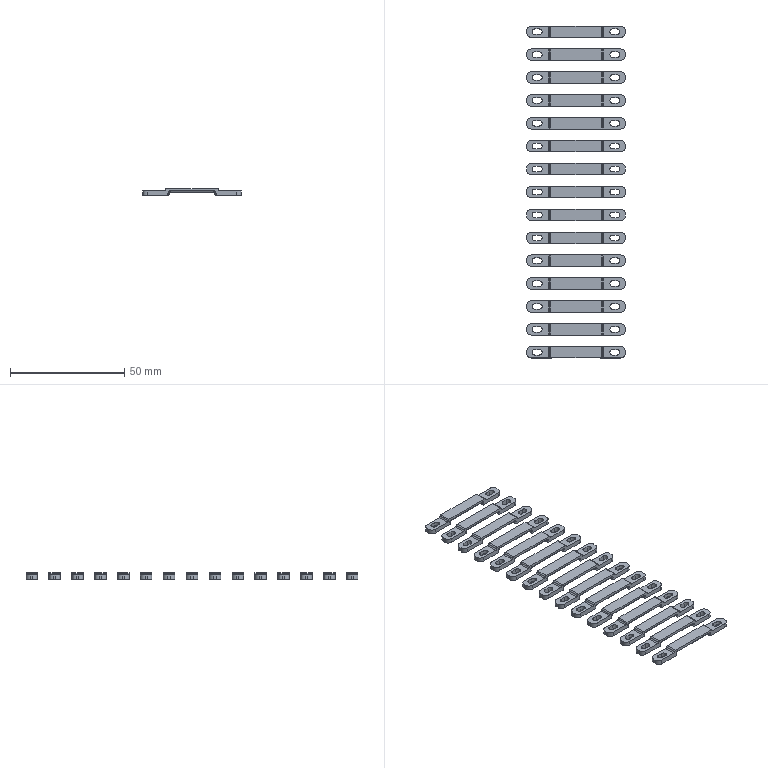NC program | NX | posted with a generic post | part box 43 x 145 x 3 mm
Lines 19 to 1188 of 17881:
(ZLEVEL_PROFILE , TOOL : D4)
N36 T11 M6
N38 G54
N40 G17 G0 G90 X65.4 Y-2.835 S9500 M3
N42 G43 Z30. H11
N44 Z1.5
N46 G94 G1 Y19.997 Z0.303 F1000.
N48 X65.787 Y21.308 Z0.232
N50 X66.58 Y22.42 Z0.16
N52 X67.692 Y23.213 Z0.089
N54 X69.003 Y23.6 Z0.017
N56 X70.997 Z-0.088
N58 X72.308 Y23.213 Z-0.159
N60 X73.42 Y22.42 Z-0.231
N62 X74.213 Y21.308 Z-0.302
N64 X74.6 Y19.997 Z-0.374
N66 Y19.5 Z-0.4
N68 Y-19.5 F2500.
N70 G2 X70.5 Y-23.6 R4.1
N72 G1 X69.5
N74 G2 X65.4 Y-19.5 R4.1
N76 G1 Y19.5
N78 G2 X69.5 Y23.6 R4.1
N80 G1 X70.5
N82 G2 X74.6 Y19.5 R4.1
N84 G1 Y-3.416 Z-0.8
N86 Y-19.5
N88 G2 X70.5 Y-23.6 R4.1
N90 G1 X69.5
N92 G2 X65.4 Y-19.5 R4.1
N94 G1 Y19.5
N96 G2 X69.5 Y23.6 R4.1
N98 G1 X70.5
N100 G2 X74.6 Y19.5 R4.1
N102 G1 Y-3.416 Z-1.2
N104 Y-19.5
N106 G2 X70.5 Y-23.6 R4.1
N108 G1 X69.5
N110 G2 X65.4 Y-19.5 R4.1
N112 G1 Y19.5
N114 G2 X69.5 Y23.6 R4.1
N116 G1 X70.5
N118 G2 X74.6 Y19.5 R4.1
N120 G1 Y-3.416 Z-1.6
N122 Y-19.5
N124 G2 X70.5 Y-23.6 R4.1
N126 G1 X69.5
N128 G2 X65.4 Y-19.5 R4.1
N130 G1 Y19.5
N132 G2 X69.5 Y23.6 R4.1
N134 G1 X70.5
N136 G2 X74.6 Y19.5 R4.1
N138 G1 Y-3.416 Z-2.
N140 Y-19.5
N142 G2 X70.5 Y-23.6 R4.1
N144 G1 X69.5
N146 G2 X65.4 Y-19.5 R4.1
N148 G1 Y19.5
N150 G2 X69.5 Y23.6 R4.1
N152 G1 X70.5
N154 G2 X74.6 Y19.5 R4.1
N156 G1 Y-3.416 Z-2.4
N158 Y-19.5
N160 G2 X70.5 Y-23.6 R4.1
N162 G1 X69.5
N164 G2 X65.4 Y-19.5 R4.1
N166 G1 Y19.5
N168 G2 X69.5 Y23.6 R4.1
N170 G1 X70.5
N172 G2 X74.6 Y19.5 R4.1
N174 G1 Y-3.416
N176 Z-0.9
N178 G0 Z30.
N180 X55.4 Y-2.835
N182 Z1.5
N184 G1 Y19.997 Z0.303 F1000.
N186 X55.787 Y21.308 Z0.232
N188 X56.58 Y22.42 Z0.16
N190 X57.692 Y23.213 Z0.089
N192 X59.003 Y23.6 Z0.017
N194 X60.997 Z-0.088
N196 X62.308 Y23.213 Z-0.159
N198 X63.42 Y22.42 Z-0.231
N200 X64.213 Y21.308 Z-0.302
N202 X64.6 Y19.997 Z-0.374
N204 Y19.5 Z-0.4
N206 Y-19.5 F2500.
N208 G2 X60.5 Y-23.6 R4.1
N210 G1 X59.5
N212 G2 X55.4 Y-19.5 R4.1
N214 G1 Y19.5
N216 G2 X59.5 Y23.6 R4.1
N218 G1 X60.5
N220 G2 X64.6 Y19.5 R4.1
N222 G1 Y-3.416 Z-0.8
N224 Y-19.5
N226 G2 X60.5 Y-23.6 R4.1
N228 G1 X59.5
N230 G2 X55.4 Y-19.5 R4.1
N232 G1 Y19.5
N234 G2 X59.5 Y23.6 R4.1
N236 G1 X60.5
N238 G2 X64.6 Y19.5 R4.1
N240 G1 Y-3.416 Z-1.2
N242 Y-19.5
N244 G2 X60.5 Y-23.6 R4.1
N246 G1 X59.5
N248 G2 X55.4 Y-19.5 R4.1
N250 G1 Y19.5
N252 G2 X59.5 Y23.6 R4.1
N254 G1 X60.5
N256 G2 X64.6 Y19.5 R4.1
N258 G1 Y-3.416 Z-1.6
N260 Y-19.5
N262 G2 X60.5 Y-23.6 R4.1
N264 G1 X59.5
N266 G2 X55.4 Y-19.5 R4.1
N268 G1 Y19.5
N270 G2 X59.5 Y23.6 R4.1
N272 G1 X60.5
N274 G2 X64.6 Y19.5 R4.1
N276 G1 Y-3.416 Z-2.
N278 Y-19.5
N280 G2 X60.5 Y-23.6 R4.1
N282 G1 X59.5
N284 G2 X55.4 Y-19.5 R4.1
N286 G1 Y19.5
N288 G2 X59.5 Y23.6 R4.1
N290 G1 X60.5
N292 G2 X64.6 Y19.5 R4.1
N294 G1 Y-3.416 Z-2.4
N296 Y-19.5
N298 G2 X60.5 Y-23.6 R4.1
N300 G1 X59.5
N302 G2 X55.4 Y-19.5 R4.1
N304 G1 Y19.5
N306 G2 X59.5 Y23.6 R4.1
N308 G1 X60.5
N310 G2 X64.6 Y19.5 R4.1
N312 G1 Y-3.416
N314 Z-0.9
N316 G0 Z30.
N318 X45.4 Y-2.835
N320 Z1.5
N322 G1 Y19.997 Z0.303 F1000.
N324 X45.787 Y21.308 Z0.232
N326 X46.58 Y22.42 Z0.16
N328 X47.692 Y23.213 Z0.089
N330 X49.003 Y23.6 Z0.017
N332 X50.997 Z-0.088
N334 X52.308 Y23.213 Z-0.159
N336 X53.42 Y22.42 Z-0.231
N338 X54.213 Y21.308 Z-0.302
N340 X54.6 Y19.997 Z-0.374
N342 Y19.5 Z-0.4
N344 Y-19.5 F2500.
N346 G2 X50.5 Y-23.6 R4.1
N348 G1 X49.5
N350 G2 X45.4 Y-19.5 R4.1
N352 G1 Y19.5
N354 G2 X49.5 Y23.6 R4.1
N356 G1 X50.5
N358 G2 X54.6 Y19.5 R4.1
N360 G1 Y-3.416 Z-0.8
N362 Y-19.5
N364 G2 X50.5 Y-23.6 R4.1
N366 G1 X49.5
N368 G2 X45.4 Y-19.5 R4.1
N370 G1 Y19.5
N372 G2 X49.5 Y23.6 R4.1
N374 G1 X50.5
N376 G2 X54.6 Y19.5 R4.1
N378 G1 Y-3.416 Z-1.2
N380 Y-19.5
N382 G2 X50.5 Y-23.6 R4.1
N384 G1 X49.5
N386 G2 X45.4 Y-19.5 R4.1
N388 G1 Y19.5
N390 G2 X49.5 Y23.6 R4.1
N392 G1 X50.5
N394 G2 X54.6 Y19.5 R4.1
N396 G1 Y-3.416 Z-1.6
N398 Y-19.5
N400 G2 X50.5 Y-23.6 R4.1
N402 G1 X49.5
N404 G2 X45.4 Y-19.5 R4.1
N406 G1 Y19.5
N408 G2 X49.5 Y23.6 R4.1
N410 G1 X50.5
N412 G2 X54.6 Y19.5 R4.1
N414 G1 Y-3.416 Z-2.
N416 Y-19.5
N418 G2 X50.5 Y-23.6 R4.1
N420 G1 X49.5
N422 G2 X45.4 Y-19.5 R4.1
N424 G1 Y19.5
N426 G2 X49.5 Y23.6 R4.1
N428 G1 X50.5
N430 G2 X54.6 Y19.5 R4.1
N432 G1 Y-3.416 Z-2.4
N434 Y-19.5
N436 G2 X50.5 Y-23.6 R4.1
N438 G1 X49.5
N440 G2 X45.4 Y-19.5 R4.1
N442 G1 Y19.5
N444 G2 X49.5 Y23.6 R4.1
N446 G1 X50.5
N448 G2 X54.6 Y19.5 R4.1
N450 G1 Y-3.416
N452 Z-0.9
N454 G0 Z30.
N456 X35.4 Y-2.835
N458 Z1.5
N460 G1 Y19.997 Z0.303 F1000.
N462 X35.787 Y21.308 Z0.232
N464 X36.58 Y22.42 Z0.16
N466 X37.692 Y23.213 Z0.089
N468 X39.003 Y23.6 Z0.017
N470 X40.997 Z-0.088
N472 X42.308 Y23.213 Z-0.159
N474 X43.42 Y22.42 Z-0.231
N476 X44.213 Y21.308 Z-0.302
N478 X44.6 Y19.997 Z-0.374
N480 Y19.5 Z-0.4
N482 Y-19.5 F2500.
N484 G2 X40.5 Y-23.6 R4.1
N486 G1 X39.5
N488 G2 X35.4 Y-19.5 R4.1
N490 G1 Y19.5
N492 G2 X39.5 Y23.6 R4.1
N494 G1 X40.5
N496 G2 X44.6 Y19.5 R4.1
N498 G1 Y-3.416 Z-0.8
N500 Y-19.5
N502 G2 X40.5 Y-23.6 R4.1
N504 G1 X39.5
N506 G2 X35.4 Y-19.5 R4.1
N508 G1 Y19.5
N510 G2 X39.5 Y23.6 R4.1
N512 G1 X40.5
N514 G2 X44.6 Y19.5 R4.1
N516 G1 Y-3.416 Z-1.2
N518 Y-19.5
N520 G2 X40.5 Y-23.6 R4.1
N522 G1 X39.5
N524 G2 X35.4 Y-19.5 R4.1
N526 G1 Y19.5
N528 G2 X39.5 Y23.6 R4.1
N530 G1 X40.5
N532 G2 X44.6 Y19.5 R4.1
N534 G1 Y-3.416 Z-1.6
N536 Y-19.5
N538 G2 X40.5 Y-23.6 R4.1
N540 G1 X39.5
N542 G2 X35.4 Y-19.5 R4.1
N544 G1 Y19.5
N546 G2 X39.5 Y23.6 R4.1
N548 G1 X40.5
N550 G2 X44.6 Y19.5 R4.1
N552 G1 Y-3.416 Z-2.
N554 Y-19.5
N556 G2 X40.5 Y-23.6 R4.1
N558 G1 X39.5
N560 G2 X35.4 Y-19.5 R4.1
N562 G1 Y19.5
N564 G2 X39.5 Y23.6 R4.1
N566 G1 X40.5
N568 G2 X44.6 Y19.5 R4.1
N570 G1 Y-3.416 Z-2.4
N572 Y-19.5
N574 G2 X40.5 Y-23.6 R4.1
N576 G1 X39.5
N578 G2 X35.4 Y-19.5 R4.1
N580 G1 Y19.5
N582 G2 X39.5 Y23.6 R4.1
N584 G1 X40.5
N586 G2 X44.6 Y19.5 R4.1
N588 G1 Y-3.416
N590 Z-0.9
N592 G0 Z30.
N594 X25.4 Y-2.835
N596 Z1.5
N598 G1 Y19.997 Z0.303 F1000.
N600 X25.787 Y21.308 Z0.232
N602 X26.58 Y22.42 Z0.16
N604 X27.692 Y23.213 Z0.089
N606 X29.003 Y23.6 Z0.017
N608 X30.997 Z-0.088
N610 X32.308 Y23.213 Z-0.159
N612 X33.42 Y22.42 Z-0.231
N614 X34.213 Y21.308 Z-0.302
N616 X34.6 Y19.997 Z-0.374
N618 Y19.5 Z-0.4
N620 Y-19.5 F2500.
N622 G2 X30.5 Y-23.6 R4.1
N624 G1 X29.5
N626 G2 X25.4 Y-19.5 R4.1
N628 G1 Y19.5
N630 G2 X29.5 Y23.6 R4.1
N632 G1 X30.5
N634 G2 X34.6 Y19.5 R4.1
N636 G1 Y-3.416 Z-0.8
N638 Y-19.5
N640 G2 X30.5 Y-23.6 R4.1
N642 G1 X29.5
N644 G2 X25.4 Y-19.5 R4.1
N646 G1 Y19.5
N648 G2 X29.5 Y23.6 R4.1
N650 G1 X30.5
N652 G2 X34.6 Y19.5 R4.1
N654 G1 Y-3.416 Z-1.2
N656 Y-19.5
N658 G2 X30.5 Y-23.6 R4.1
N660 G1 X29.5
N662 G2 X25.4 Y-19.5 R4.1
N664 G1 Y19.5
N666 G2 X29.5 Y23.6 R4.1
N668 G1 X30.5
N670 G2 X34.6 Y19.5 R4.1
N672 G1 Y-3.416 Z-1.6
N674 Y-19.5
N676 G2 X30.5 Y-23.6 R4.1
N678 G1 X29.5
N680 G2 X25.4 Y-19.5 R4.1
N682 G1 Y19.5
N684 G2 X29.5 Y23.6 R4.1
N686 G1 X30.5
N688 G2 X34.6 Y19.5 R4.1
N690 G1 Y-3.416 Z-2.
N692 Y-19.5
N694 G2 X30.5 Y-23.6 R4.1
N696 G1 X29.5
N698 G2 X25.4 Y-19.5 R4.1
N700 G1 Y19.5
N702 G2 X29.5 Y23.6 R4.1
N704 G1 X30.5
N706 G2 X34.6 Y19.5 R4.1
N708 G1 Y-3.416 Z-2.4
N710 Y-19.5
N712 G2 X30.5 Y-23.6 R4.1
N714 G1 X29.5
N716 G2 X25.4 Y-19.5 R4.1
N718 G1 Y19.5
N720 G2 X29.5 Y23.6 R4.1
N722 G1 X30.5
N724 G2 X34.6 Y19.5 R4.1
N726 G1 Y-3.416
N728 Z-0.9
N730 G0 Z30.
N732 X-44.6 Y-2.835
N734 Z1.5
N736 G1 Y19.997 Z0.303 F1000.
N738 X-44.213 Y21.308 Z0.232
N740 X-43.42 Y22.42 Z0.16
N742 X-42.308 Y23.213 Z0.089
N744 X-40.997 Y23.6 Z0.017
N746 X-39.003 Z-0.088
N748 X-37.692 Y23.213 Z-0.159
N750 X-36.58 Y22.42 Z-0.231
N752 X-35.787 Y21.308 Z-0.302
N754 X-35.4 Y19.997 Z-0.374
N756 Y19.5 Z-0.4
N758 Y-19.5 F2500.
N760 G2 X-39.5 Y-23.6 R4.1
N762 G1 X-40.5
N764 G2 X-44.6 Y-19.5 R4.1
N766 G1 Y19.5
N768 G2 X-40.5 Y23.6 R4.1
N770 G1 X-39.5
N772 G2 X-35.4 Y19.5 R4.1
N774 G1 Y-3.416 Z-0.8
N776 Y-19.5
N778 G2 X-39.5 Y-23.6 R4.1
N780 G1 X-40.5
N782 G2 X-44.6 Y-19.5 R4.1
N784 G1 Y19.5
N786 G2 X-40.5 Y23.6 R4.1
N788 G1 X-39.5
N790 G2 X-35.4 Y19.5 R4.1
N792 G1 Y-3.416 Z-1.2
N794 Y-19.5
N796 G2 X-39.5 Y-23.6 R4.1
N798 G1 X-40.5
N800 G2 X-44.6 Y-19.5 R4.1
N802 G1 Y19.5
N804 G2 X-40.5 Y23.6 R4.1
N806 G1 X-39.5
N808 G2 X-35.4 Y19.5 R4.1
N810 G1 Y-3.416 Z-1.6
N812 Y-19.5
N814 G2 X-39.5 Y-23.6 R4.1
N816 G1 X-40.5
N818 G2 X-44.6 Y-19.5 R4.1
N820 G1 Y19.5
N822 G2 X-40.5 Y23.6 R4.1
N824 G1 X-39.5
N826 G2 X-35.4 Y19.5 R4.1
N828 G1 Y-3.416 Z-2.
N830 Y-19.5
N832 G2 X-39.5 Y-23.6 R4.1
N834 G1 X-40.5
N836 G2 X-44.6 Y-19.5 R4.1
N838 G1 Y19.5
N840 G2 X-40.5 Y23.6 R4.1
N842 G1 X-39.5
N844 G2 X-35.4 Y19.5 R4.1
N846 G1 Y-3.416 Z-2.4
N848 Y-19.5
N850 G2 X-39.5 Y-23.6 R4.1
N852 G1 X-40.5
N854 G2 X-44.6 Y-19.5 R4.1
N856 G1 Y19.5
N858 G2 X-40.5 Y23.6 R4.1
N860 G1 X-39.5
N862 G2 X-35.4 Y19.5 R4.1
N864 G1 Y-3.416
N866 Z-0.9
N868 G0 Z30.
N870 X-55.4 Y2.835
N872 Z1.5
N874 G1 Y-19.997 Z0.303 F1000.
N876 X-55.787 Y-21.308 Z0.232
N878 X-56.58 Y-22.42 Z0.16
N880 X-57.692 Y-23.213 Z0.089
N882 X-59.003 Y-23.6 Z0.017
N884 X-60.997 Z-0.088
N886 X-62.308 Y-23.213 Z-0.159
N888 X-63.42 Y-22.42 Z-0.231
N890 X-64.213 Y-21.308 Z-0.302
N892 X-64.6 Y-19.997 Z-0.374
N894 Y-19.5 Z-0.4
N896 Y19.5 F2500.
N898 G2 X-60.5 Y23.6 R4.1
N900 G1 X-59.5
N902 G2 X-55.4 Y19.5 R4.1
N904 G1 Y-19.5
N906 G2 X-59.5 Y-23.6 R4.1
N908 G1 X-60.5
N910 G2 X-64.6 Y-19.5 R4.1
N912 G1 Y3.416 Z-0.8
N914 Y19.5
N916 G2 X-60.5 Y23.6 R4.1
N918 G1 X-59.5
N920 G2 X-55.4 Y19.5 R4.1
N922 G1 Y-19.5
N924 G2 X-59.5 Y-23.6 R4.1
N926 G1 X-60.5
N928 G2 X-64.6 Y-19.5 R4.1
N930 G1 Y3.416 Z-1.2
N932 Y19.5
N934 G2 X-60.5 Y23.6 R4.1
N936 G1 X-59.5
N938 G2 X-55.4 Y19.5 R4.1
N940 G1 Y-19.5
N942 G2 X-59.5 Y-23.6 R4.1
N944 G1 X-60.5
N946 G2 X-64.6 Y-19.5 R4.1
N948 G1 Y3.416 Z-1.6
N950 Y19.5
N952 G2 X-60.5 Y23.6 R4.1
N954 G1 X-59.5
N956 G2 X-55.4 Y19.5 R4.1
N958 G1 Y-19.5
N960 G2 X-59.5 Y-23.6 R4.1
N962 G1 X-60.5
N964 G2 X-64.6 Y-19.5 R4.1
N966 G1 Y3.416 Z-2.
N968 Y19.5
N970 G2 X-60.5 Y23.6 R4.1
N972 G1 X-59.5
N974 G2 X-55.4 Y19.5 R4.1
N976 G1 Y-19.5
N978 G2 X-59.5 Y-23.6 R4.1
N980 G1 X-60.5
N982 G2 X-64.6 Y-19.5 R4.1
N984 G1 Y3.416 Z-2.4
N986 Y19.5
N988 G2 X-60.5 Y23.6 R4.1
N990 G1 X-59.5
N992 G2 X-55.4 Y19.5 R4.1
N994 G1 Y-19.5
N996 G2 X-59.5 Y-23.6 R4.1
N998 G1 X-60.5
N1000 G2 X-64.6 Y-19.5 R4.1
N1002 G1 Y3.416
N1004 Z-0.9
N1006 G0 Z30.
N1008 X24.6 Y2.835
N1010 Z1.5
N1012 G1 Y-19.997 Z0.303 F1000.
N1014 X24.213 Y-21.308 Z0.232
N1016 X23.42 Y-22.42 Z0.16
N1018 X22.308 Y-23.213 Z0.089
N1020 X20.997 Y-23.6 Z0.017
N1022 X19.003 Z-0.088
N1024 X17.692 Y-23.213 Z-0.159
N1026 X16.58 Y-22.42 Z-0.231
N1028 X15.787 Y-21.308 Z-0.302
N1030 X15.4 Y-19.997 Z-0.374
N1032 Y-19.5 Z-0.4
N1034 Y19.5 F2500.
N1036 G2 X19.5 Y23.6 R4.1
N1038 G1 X20.5
N1040 G2 X24.6 Y19.5 R4.1
N1042 G1 Y-19.5
N1044 G2 X20.5 Y-23.6 R4.1
N1046 G1 X19.5
N1048 G2 X15.4 Y-19.5 R4.1
N1050 G1 Y3.416 Z-0.8
N1052 Y19.5
N1054 G2 X19.5 Y23.6 R4.1
N1056 G1 X20.5
N1058 G2 X24.6 Y19.5 R4.1
N1060 G1 Y-19.5
N1062 G2 X20.5 Y-23.6 R4.1
N1064 G1 X19.5
N1066 G2 X15.4 Y-19.5 R4.1
N1068 G1 Y3.416 Z-1.2
N1070 Y19.5
N1072 G2 X19.5 Y23.6 R4.1
N1074 G1 X20.5
N1076 G2 X24.6 Y19.5 R4.1
N1078 G1 Y-19.5
N1080 G2 X20.5 Y-23.6 R4.1
N1082 G1 X19.5
N1084 G2 X15.4 Y-19.5 R4.1
N1086 G1 Y3.416 Z-1.6
N1088 Y19.5
N1090 G2 X19.5 Y23.6 R4.1
N1092 G1 X20.5
N1094 G2 X24.6 Y19.5 R4.1
N1096 G1 Y-19.5
N1098 G2 X20.5 Y-23.6 R4.1
N1100 G1 X19.5
N1102 G2 X15.4 Y-19.5 R4.1
N1104 G1 Y3.416 Z-2.
N1106 Y19.5
N1108 G2 X19.5 Y23.6 R4.1
N1110 G1 X20.5
N1112 G2 X24.6 Y19.5 R4.1
N1114 G1 Y-19.5
N1116 G2 X20.5 Y-23.6 R4.1
N1118 G1 X19.5
N1120 G2 X15.4 Y-19.5 R4.1
N1122 G1 Y3.416 Z-2.4
N1124 Y19.5
N1126 G2 X19.5 Y23.6 R4.1
N1128 G1 X20.5
N1130 G2 X24.6 Y19.5 R4.1
N1132 G1 Y-19.5
N1134 G2 X20.5 Y-23.6 R4.1
N1136 G1 X19.5
N1138 G2 X15.4 Y-19.5 R4.1
N1140 G1 Y3.416
N1142 Z-0.9
N1144 G0 Z30.
N1146 X-65.4 Y2.835
N1148 Z1.5
N1150 G1 Y-19.997 Z0.303 F1000.
N1152 X-65.787 Y-21.308 Z0.232
N1154 X-66.58 Y-22.42 Z0.16
N1156 X-67.692 Y-23.213 Z0.089
N1158 X-69.003 Y-23.6 Z0.017
N1160 X-70.997 Z-0.088
N1162 X-72.308 Y-23.213 Z-0.159
N1164 X-73.42 Y-22.42 Z-0.231
N1166 X-74.213 Y-21.308 Z-0.302
N1168 X-74.6 Y-19.997 Z-0.374
N1170 Y-19.5 Z-0.4
N1172 Y19.5 F2500.
N1174 G2 X-70.5 Y23.6 R4.1
N1176 G1 X-69.5
N1178 G2 X-65.4 Y19.5 R4.1
N1180 G1 Y-19.5
N1182 G2 X-69.5 Y-23.6 R4.1
N1184 G1 X-70.5
N1186 G2 X-74.6 Y-19.5 R4.1
N1188 G1 Y3.416 Z-0.8
N1190 Y19.5
N1192 G2 X-70.5 Y23.6 R4.1
N1194 G1 X-69.5
N1196 G2 X-65.4 Y19.5 R4.1
N1198 G1 Y-19.5
N1200 G2 X-69.5 Y-23.6 R4.1
N1202 G1 X-70.5
N1204 G2 X-74.6 Y-19.5 R4.1
N1206 G1 Y3.416 Z-1.2
N1208 Y19.5
N1210 G2 X-70.5 Y23.6 R4.1
N1212 G1 X-69.5
N1214 G2 X-65.4 Y19.5 R4.1
N1216 G1 Y-19.5
N1218 G2 X-69.5 Y-23.6 R4.1
N1220 G1 X-70.5
N1222 G2 X-74.6 Y-19.5 R4.1
N1224 G1 Y3.416 Z-1.6
N1226 Y19.5
N1228 G2 X-70.5 Y23.6 R4.1
N1230 G1 X-69.5
N1232 G2 X-65.4 Y19.5 R4.1
N1234 G1 Y-19.5
N1236 G2 X-69.5 Y-23.6 R4.1
N1238 G1 X-70.5
N1240 G2 X-74.6 Y-19.5 R4.1
N1242 G1 Y3.416 Z-2.
N1244 Y19.5
N1246 G2 X-70.5 Y23.6 R4.1
N1248 G1 X-69.5
N1250 G2 X-65.4 Y19.5 R4.1
N1252 G1 Y-19.5
N1254 G2 X-69.5 Y-23.6 R4.1
N1256 G1 X-70.5
N1258 G2 X-74.6 Y-19.5 R4.1
N1260 G1 Y3.416 Z-2.4
N1262 Y19.5
N1264 G2 X-70.5 Y23.6 R4.1
N1266 G1 X-69.5
N1268 G2 X-65.4 Y19.5 R4.1
N1270 G1 Y-19.5
N1272 G2 X-69.5 Y-23.6 R4.1
N1274 G1 X-70.5
N1276 G2 X-74.6 Y-19.5 R4.1
N1278 G1 Y3.416
N1280 Z-0.9
N1282 G0 Z30.
N1284 X14.6 Y2.835
N1286 Z1.5
N1288 G1 Y-19.997 Z0.303 F1000.
N1290 X14.213 Y-21.308 Z0.232
N1292 X13.42 Y-22.42 Z0.16
N1294 X12.308 Y-23.213 Z0.089
N1296 X10.997 Y-23.6 Z0.017
N1298 X9.003 Z-0.088
N1300 X7.692 Y-23.213 Z-0.159
N1302 X6.58 Y-22.42 Z-0.231
N1304 X5.787 Y-21.308 Z-0.302
N1306 X5.4 Y-19.997 Z-0.374
N1308 Y-19.5 Z-0.4
N1310 Y19.5 F2500.
N1312 G2 X9.5 Y23.6 R4.1
N1314 G1 X10.5
N1316 G2 X14.6 Y19.5 R4.1
N1318 G1 Y-19.5
N1320 G2 X10.5 Y-23.6 R4.1
N1322 G1 X9.5
N1324 G2 X5.4 Y-19.5 R4.1
N1326 G1 Y3.416 Z-0.8
N1328 Y19.5
N1330 G2 X9.5 Y23.6 R4.1
N1332 G1 X10.5
N1334 G2 X14.6 Y19.5 R4.1
N1336 G1 Y-19.5
N1338 G2 X10.5 Y-23.6 R4.1
N1340 G1 X9.5
N1342 G2 X5.4 Y-19.5 R4.1
N1344 G1 Y3.416 Z-1.2
N1346 Y19.5
N1348 G2 X9.5 Y23.6 R4.1
N1350 G1 X10.5
N1352 G2 X14.6 Y19.5 R4.1
N1354 G1 Y-19.5
N1356 G2 X10.5 Y-23.6 R4.1
N1358 G1 X9.5
N1360 G2 X5.4 Y-19.5 R4.1
N1362 G1 Y3.416 Z-1.6
N1364 Y19.5
N1366 G2 X9.5 Y23.6 R4.1
N1368 G1 X10.5
N1370 G2 X14.6 Y19.5 R4.1
N1372 G1 Y-19.5
N1374 G2 X10.5 Y-23.6 R4.1
N1376 G1 X9.5
N1378 G2 X5.4 Y-19.5 R4.1
N1380 G1 Y3.416 Z-2.
N1382 Y19.5
N1384 G2 X9.5 Y23.6 R4.1
N1386 G1 X10.5
N1388 G2 X14.6 Y19.5 R4.1
N1390 G1 Y-19.5
N1392 G2 X10.5 Y-23.6 R4.1
N1394 G1 X9.5
N1396 G2 X5.4 Y-19.5 R4.1
N1398 G1 Y3.416 Z-2.4
N1400 Y19.5
N1402 G2 X9.5 Y23.6 R4.1
N1404 G1 X10.5
N1406 G2 X14.6 Y19.5 R4.1
N1408 G1 Y-19.5
N1410 G2 X10.5 Y-23.6 R4.1
N1412 G1 X9.5
N1414 G2 X5.4 Y-19.5 R4.1
N1416 G1 Y3.416
N1418 Z-0.9
N1420 G0 Z30.
N1422 X-4.6 Y-2.835
N1424 Z1.5
N1426 G1 Y19.997 Z0.303 F1000.
N1428 X-4.213 Y21.308 Z0.232
N1430 X-3.42 Y22.42 Z0.16
N1432 X-2.308 Y23.213 Z0.089
N1434 X-0.997 Y23.6 Z0.017
N1436 X0.997 Z-0.088
N1438 X2.308 Y23.213 Z-0.159
N1440 X3.42 Y22.42 Z-0.231
N1442 X4.213 Y21.308 Z-0.302
N1444 X4.6 Y19.997 Z-0.374
N1446 Y19.5 Z-0.4
N1448 Y-19.5 F2500.
N1450 G2 X0.5 Y-23.6 R4.1
N1452 G1 X-0.5
N1454 G2 X-4.6 Y-19.5 R4.1
N1456 G1 Y19.5
N1458 G2 X-0.5 Y23.6 R4.1
N1460 G1 X0.5
N1462 G2 X4.6 Y19.5 R4.1
N1464 G1 Y-3.416 Z-0.8
N1466 Y-19.5
N1468 G2 X0.5 Y-23.6 R4.1
N1470 G1 X-0.5
N1472 G2 X-4.6 Y-19.5 R4.1
N1474 G1 Y19.5
N1476 G2 X-0.5 Y23.6 R4.1
N1478 G1 X0.5
N1480 G2 X4.6 Y19.5 R4.1
N1482 G1 Y-3.416 Z-1.2
N1484 Y-19.5
N1486 G2 X0.5 Y-23.6 R4.1
N1488 G1 X-0.5
N1490 G2 X-4.6 Y-19.5 R4.1
N1492 G1 Y19.5
N1494 G2 X-0.5 Y23.6 R4.1
N1496 G1 X0.5
N1498 G2 X4.6 Y19.5 R4.1
N1500 G1 Y-3.416 Z-1.6
N1502 Y-19.5
N1504 G2 X0.5 Y-23.6 R4.1
N1506 G1 X-0.5
N1508 G2 X-4.6 Y-19.5 R4.1
N1510 G1 Y19.5
N1512 G2 X-0.5 Y23.6 R4.1
N1514 G1 X0.5
N1516 G2 X4.6 Y19.5 R4.1
N1518 G1 Y-3.416 Z-2.
N1520 Y-19.5
N1522 G2 X0.5 Y-23.6 R4.1
N1524 G1 X-0.5
N1526 G2 X-4.6 Y-19.5 R4.1
N1528 G1 Y19.5
N1530 G2 X-0.5 Y23.6 R4.1
N1532 G1 X0.5
N1534 G2 X4.6 Y19.5 R4.1
N1536 G1 Y-3.416 Z-2.4
N1538 Y-19.5
N1540 G2 X0.5 Y-23.6 R4.1
N1542 G1 X-0.5
N1544 G2 X-4.6 Y-19.5 R4.1
N1546 G1 Y19.5
N1548 G2 X-0.5 Y23.6 R4.1
N1550 G1 X0.5
N1552 G2 X4.6 Y19.5 R4.1
N1554 G1 Y-3.416
N1556 Z-0.9
N1558 G0 Z30.
N1560 X-14.6 Y-2.835
N1562 Z1.5
N1564 G1 Y19.997 Z0.303 F1000.
N1566 X-14.213 Y21.308 Z0.232
N1568 X-13.42 Y22.42 Z0.16
N1570 X-12.308 Y23.213 Z0.089
N1572 X-10.997 Y23.6 Z0.017
N1574 X-9.003 Z-0.088
N1576 X-7.692 Y23.213 Z-0.159
N1578 X-6.58 Y22.42 Z-0.231
N1580 X-5.787 Y21.308 Z-0.302
N1582 X-5.4 Y19.997 Z-0.374
N1584 Y19.5 Z-0.4
N1586 Y-19.5 F2500.
N1588 G2 X-9.5 Y-23.6 R4.1
N1590 G1 X-10.5
N1592 G2 X-14.6 Y-19.5 R4.1
N1594 G1 Y19.5
N1596 G2 X-10.5 Y23.6 R4.1
N1598 G1 X-9.5
N1600 G2 X-5.4 Y19.5 R4.1
N1602 G1 Y-3.416 Z-0.8
N1604 Y-19.5
N1606 G2 X-9.5 Y-23.6 R4.1
N1608 G1 X-10.5
N1610 G2 X-14.6 Y-19.5 R4.1
N1612 G1 Y19.5
N1614 G2 X-10.5 Y23.6 R4.1
N1616 G1 X-9.5
N1618 G2 X-5.4 Y19.5 R4.1
N1620 G1 Y-3.416 Z-1.2
N1622 Y-19.5
N1624 G2 X-9.5 Y-23.6 R4.1
N1626 G1 X-10.5
N1628 G2 X-14.6 Y-19.5 R4.1
N1630 G1 Y19.5
N1632 G2 X-10.5 Y23.6 R4.1
N1634 G1 X-9.5
N1636 G2 X-5.4 Y19.5 R4.1
N1638 G1 Y-3.416 Z-1.6
N1640 Y-19.5
N1642 G2 X-9.5 Y-23.6 R4.1
N1644 G1 X-10.5
N1646 G2 X-14.6 Y-19.5 R4.1
N1648 G1 Y19.5
N1650 G2 X-10.5 Y23.6 R4.1
N1652 G1 X-9.5
N1654 G2 X-5.4 Y19.5 R4.1
N1656 G1 Y-3.416 Z-2.
N1658 Y-19.5
N1660 G2 X-9.5 Y-23.6 R4.1
N1662 G1 X-10.5
N1664 G2 X-14.6 Y-19.5 R4.1
N1666 G1 Y19.5
N1668 G2 X-10.5 Y23.6 R4.1
N1670 G1 X-9.5
N1672 G2 X-5.4 Y19.5 R4.1
N1674 G1 Y-3.416 Z-2.4
N1676 Y-19.5
N1678 G2 X-9.5 Y-23.6 R4.1
N1680 G1 X-10.5
N1682 G2 X-14.6 Y-19.5 R4.1
N1684 G1 Y19.5
N1686 G2 X-10.5 Y23.6 R4.1
N1688 G1 X-9.5
N1690 G2 X-5.4 Y19.5 R4.1
N1692 G1 Y-3.416
N1694 Z-0.9
N1696 G0 Z30.
N1698 X-24.6 Y-2.835
N1700 Z1.5
N1702 G1 Y19.997 Z0.303 F1000.
N1704 X-24.213 Y21.308 Z0.232
N1706 X-23.42 Y22.42 Z0.16
N1708 X-22.308 Y23.213 Z0.089
N1710 X-20.997 Y23.6 Z0.017
N1712 X-19.003 Z-0.088
N1714 X-17.692 Y23.213 Z-0.159
N1716 X-16.58 Y22.42 Z-0.231
N1718 X-15.787 Y21.308 Z-0.302
N1720 X-15.4 Y19.997 Z-0.374
N1722 Y19.5 Z-0.4
N1724 Y-19.5 F2500.
N1726 G2 X-19.5 Y-23.6 R4.1
N1728 G1 X-20.5
N1730 G2 X-24.6 Y-19.5 R4.1
N1732 G1 Y19.5
N1734 G2 X-20.5 Y23.6 R4.1
N1736 G1 X-19.5
N1738 G2 X-15.4 Y19.5 R4.1
N1740 G1 Y-3.416 Z-0.8
N1742 Y-19.5
N1744 G2 X-19.5 Y-23.6 R4.1
N1746 G1 X-20.5
N1748 G2 X-24.6 Y-19.5 R4.1
N1750 G1 Y19.5
N1752 G2 X-20.5 Y23.6 R4.1
N1754 G1 X-19.5
N1756 G2 X-15.4 Y19.5 R4.1
N1758 G1 Y-3.416 Z-1.2
N1760 Y-19.5
N1762 G2 X-19.5 Y-23.6 R4.1
N1764 G1 X-20.5
N1766 G2 X-24.6 Y-19.5 R4.1
N1768 G1 Y19.5
N1770 G2 X-20.5 Y23.6 R4.1
N1772 G1 X-19.5
N1774 G2 X-15.4 Y19.5 R4.1
N1776 G1 Y-3.416 Z-1.6
N1778 Y-19.5
N1780 G2 X-19.5 Y-23.6 R4.1
N1782 G1 X-20.5
N1784 G2 X-24.6 Y-19.5 R4.1
N1786 G1 Y19.5
N1788 G2 X-20.5 Y23.6 R4.1
N1790 G1 X-19.5
N1792 G2 X-15.4 Y19.5 R4.1
N1794 G1 Y-3.416 Z-2.
N1796 Y-19.5
N1798 G2 X-19.5 Y-23.6 R4.1
N1800 G1 X-20.5
N1802 G2 X-24.6 Y-19.5 R4.1
N1804 G1 Y19.5
N1806 G2 X-20.5 Y23.6 R4.1
N1808 G1 X-19.5
N1810 G2 X-15.4 Y19.5 R4.1
N1812 G1 Y-3.416 Z-2.4
N1814 Y-19.5
N1816 G2 X-19.5 Y-23.6 R4.1
N1818 G1 X-20.5
N1820 G2 X-24.6 Y-19.5 R4.1
N1822 G1 Y19.5
N1824 G2 X-20.5 Y23.6 R4.1
N1826 G1 X-19.5
N1828 G2 X-15.4 Y19.5 R4.1
N1830 G1 Y-3.416
N1832 Z-0.9
N1834 G0 Z30.
N1836 X-34.6 Y-2.835
N1838 Z1.5
N1840 G1 Y19.997 Z0.303 F1000.
N1842 X-34.213 Y21.308 Z0.232
N1844 X-33.42 Y22.42 Z0.16
N1846 X-32.308 Y23.213 Z0.089
N1848 X-30.997 Y23.6 Z0.017
N1850 X-29.003 Z-0.088
N1852 X-27.692 Y23.213 Z-0.159
N1854 X-26.58 Y22.42 Z-0.231
N1856 X-25.787 Y21.308 Z-0.302
N1858 X-25.4 Y19.997 Z-0.374
N1860 Y19.5 Z-0.4
N1862 Y-19.5 F2500.
N1864 G2 X-29.5 Y-23.6 R4.1
N1866 G1 X-30.5
N1868 G2 X-34.6 Y-19.5 R4.1
N1870 G1 Y19.5
N1872 G2 X-30.5 Y23.6 R4.1
N1874 G1 X-29.5
N1876 G2 X-25.4 Y19.5 R4.1
N1878 G1 Y-3.416 Z-0.8
N1880 Y-19.5
N1882 G2 X-29.5 Y-23.6 R4.1
N1884 G1 X-30.5
N1886 G2 X-34.6 Y-19.5 R4.1
N1888 G1 Y19.5
N1890 G2 X-30.5 Y23.6 R4.1
N1892 G1 X-29.5
N1894 G2 X-25.4 Y19.5 R4.1
N1896 G1 Y-3.416 Z-1.2
N1898 Y-19.5
N1900 G2 X-29.5 Y-23.6 R4.1
N1902 G1 X-30.5
N1904 G2 X-34.6 Y-19.5 R4.1
N1906 G1 Y19.5
N1908 G2 X-30.5 Y23.6 R4.1
N1910 G1 X-29.5
N1912 G2 X-25.4 Y19.5 R4.1
N1914 G1 Y-3.416 Z-1.6
N1916 Y-19.5
N1918 G2 X-29.5 Y-23.6 R4.1
N1920 G1 X-30.5
N1922 G2 X-34.6 Y-19.5 R4.1
N1924 G1 Y19.5
N1926 G2 X-30.5 Y23.6 R4.1
N1928 G1 X-29.5
N1930 G2 X-25.4 Y19.5 R4.1
N1932 G1 Y-3.416 Z-2.
N1934 Y-19.5
N1936 G2 X-29.5 Y-23.6 R4.1
N1938 G1 X-30.5
N1940 G2 X-34.6 Y-19.5 R4.1
N1942 G1 Y19.5
N1944 G2 X-30.5 Y23.6 R4.1
N1946 G1 X-29.5
N1948 G2 X-25.4 Y19.5 R4.1
N1950 G1 Y-3.416 Z-2.4
N1952 Y-19.5
N1954 G2 X-29.5 Y-23.6 R4.1
N1956 G1 X-30.5
N1958 G2 X-34.6 Y-19.5 R4.1
N1960 G1 Y19.5
N1962 G2 X-30.5 Y23.6 R4.1
N1964 G1 X-29.5
N1966 G2 X-25.4 Y19.5 R4.1
N1968 G1 Y-3.416
N1970 Z-0.9
N1972 G0 Z30.
N1974 X-54.6 Y-2.835
N1976 Z1.5
N1978 G1 Y19.997 Z0.303 F1000.
N1980 X-54.213 Y21.308 Z0.232
N1982 X-53.42 Y22.42 Z0.16
N1984 X-52.308 Y23.213 Z0.089
N1986 X-50.997 Y23.6 Z0.017
N1988 X-49.003 Z-0.088
N1990 X-47.692 Y23.213 Z-0.159
N1992 X-46.58 Y22.42 Z-0.231
N1994 X-45.787 Y21.308 Z-0.302
N1996 X-45.4 Y19.997 Z-0.374
N1998 Y19.5 Z-0.4
N2000 Y-19.5 F2500.
N2002 G2 X-49.5 Y-23.6 R4.1
N2004 G1 X-50.5
N2006 G2 X-54.6 Y-19.5 R4.1
N2008 G1 Y19.5
N2010 G2 X-50.5 Y23.6 R4.1
N2012 G1 X-49.5
N2014 G2 X-45.4 Y19.5 R4.1
N2016 G1 Y-3.416 Z-0.8
N2018 Y-19.5
N2020 G2 X-49.5 Y-23.6 R4.1
N2022 G1 X-50.5
N2024 G2 X-54.6 Y-19.5 R4.1
N2026 G1 Y19.5
N2028 G2 X-50.5 Y23.6 R4.1
N2030 G1 X-49.5
N2032 G2 X-45.4 Y19.5 R4.1
N2034 G1 Y-3.416 Z-1.2
N2036 Y-19.5
N2038 G2 X-49.5 Y-23.6 R4.1
N2040 G1 X-50.5
N2042 G2 X-54.6 Y-19.5 R4.1
N2044 G1 Y19.5
N2046 G2 X-50.5 Y23.6 R4.1
N2048 G1 X-49.5
N2050 G2 X-45.4 Y19.5 R4.1
N2052 G1 Y-3.416 Z-1.6
N2054 Y-19.5
N2056 G2 X-49.5 Y-23.6 R4.1
N2058 G1 X-50.5
N2060 G2 X-54.6 Y-19.5 R4.1
N2062 G1 Y19.5
N2064 G2 X-50.5 Y23.6 R4.1
N2066 G1 X-49.5
N2068 G2 X-45.4 Y19.5 R4.1
N2070 G1 Y-3.416 Z-2.
N2072 Y-19.5
N2074 G2 X-49.5 Y-23.6 R4.1
N2076 G1 X-50.5
N2078 G2 X-54.6 Y-19.5 R4.1
N2080 G1 Y19.5
N2082 G2 X-50.5 Y23.6 R4.1
N2084 G1 X-49.5
N2086 G2 X-45.4 Y19.5 R4.1
N2088 G1 Y-3.416 Z-2.4
N2090 Y-19.5
N2092 G2 X-49.5 Y-23.6 R4.1
N2094 G1 X-50.5
N2096 G2 X-54.6 Y-19.5 R4.1
N2098 G1 Y19.5
N2100 G2 X-50.5 Y23.6 R4.1
N2102 G1 X-49.5
N2104 G2 X-45.4 Y19.5 R4.1
N2106 G1 Y-3.416
N2108 Z-0.9
N2110 G0 Z30.
(FLOOR_WALL_1 , TOOL : D4)
N2112 X75.268 Y-8.986
N2114 Z0.96
N2116 G1 Z-0.04 F1000.
N2118 X74.306 Y-7.84
N2120 G3 X74. Y-7.697 R0.4
N2122 G1 X66. F2500.
N2124 Y-5.131
N2126 X74.
N2128 Y-2.565
N2130 X66.
N2132 Y0.001
N2134 X74.
N2136 Y2.568
N2138 X66.
N2140 Y5.134
N2142 X74.
N2144 Y7.7
N2146 X66.
N2148 G3 X65.694 Y7.557 R0.4
N2150 G1 X65. Y6.731
N2152 Z0.96
N2154 G0 X75.264 Y-8.981 Z0.62
N2156 G1 Z-0.38 F1000.
N2158 X74.306 Y-7.84
N2160 G3 X74. Y-7.697 R0.4
N2162 G1 X66. F2500.
N2164 Y-5.131
N2166 X74.
N2168 Y-2.565
N2170 X66.
N2172 Y0.001
N2174 X74.
N2176 Y2.568
N2178 X66.
N2180 Y5.134
N2182 X74.
N2184 Y7.7
N2186 X66.
N2188 G3 X65.694 Y7.557 R0.4
N2190 G1 X65. Y6.731
N2192 Z0.62
N2194 G0 Z30.
N2196 X75.264 Y-8.981
N2198 Z0.28
N2200 G1 Z-0.72 F1000.
N2202 X74.306 Y-7.84
N2204 G3 X74. Y-7.697 R0.4
N2206 G1 X66. F2500.
N2208 Y-5.131
N2210 X74.
N2212 Y-2.565
N2214 X66.
N2216 Y0.001
N2218 X74.
N2220 Y2.568
N2222 X66.
N2224 Y5.134
N2226 X74.
N2228 Y7.7
N2230 X66.
N2232 G3 X65.694 Y7.557 R0.4
N2234 G1 X65. Y6.731
N2236 Z0.28
N2238 G0 Z30.
N2240 X75.268 Y-8.985
N2242 Z-0.06
N2244 G1 Z-1.06 F1000.
N2246 X74.306 Y-7.84
N2248 G3 X74. Y-7.697 R0.4
N2250 G1 X66. F2500.
N2252 Y-5.131
N2254 X74.
N2256 Y-2.565
N2258 X66.
N2260 Y0.001
N2262 X74.
N2264 Y2.568
N2266 X66.
N2268 Y5.134
N2270 X74.
N2272 Y7.7
N2274 X66.
N2276 G3 X65.694 Y7.557 R0.4
N2278 G1 X65. Y6.731
N2280 Z-0.06
N2282 G0 Z30.
N2284 X68.999 Y-7.697
N2286 Z-0.06
N2288 G1 X74. Z-1.4 F1000.
N2290 X66. F2500.
N2292 Y-5.131
N2294 X74.
N2296 Y-2.565
N2298 X66.
N2300 Y0.001
N2302 X74.
N2304 Y2.568
N2306 X66.
N2308 Y5.134
N2310 X74.
N2312 Y7.7
N2314 X66.
N2316 Z-0.4
N2318 G0 Z30.
N2320 X65. Y-7.84
N2322 Z0.96
N2324 G1 Z-0.04 F1000.
N2326 X64.306
N2328 G3 X64. Y-7.697 R0.4
N2330 G1 X56. F2500.
N2332 Y-5.131
N2334 X64.
N2336 Y-2.565
N2338 X56.
N2340 Y0.001
N2342 X64.
N2344 Y2.568
N2346 X56.
N2348 Y5.134
N2350 X64.
N2352 Y7.7
N2354 X56.
N2356 G3 X55.694 Y7.557 R0.4
N2358 G1 X55. Y6.731
N2360 Z0.96
N2362 G0 X65. Y-7.84 Z0.62